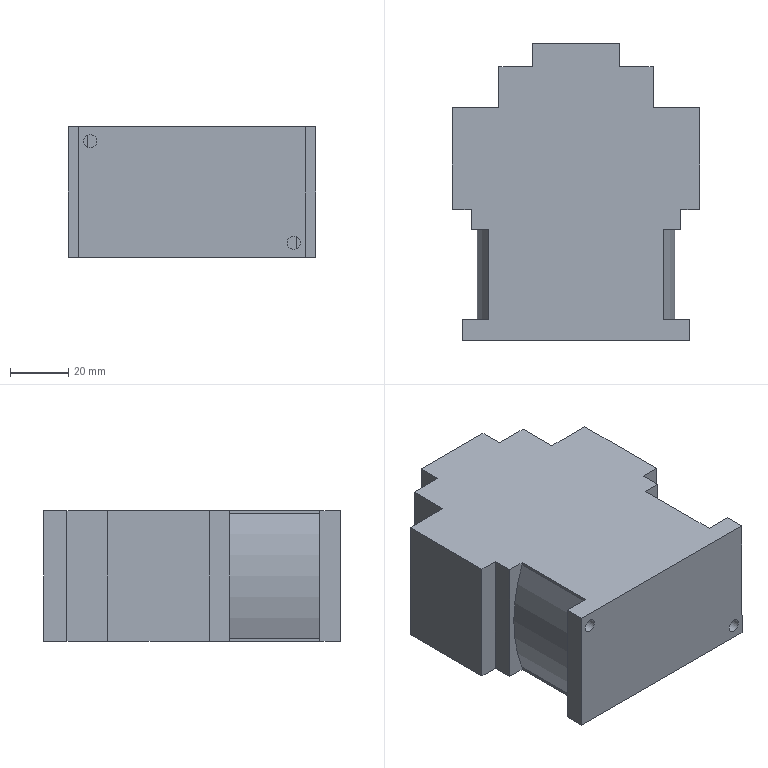Part | NX | features BREP 1 | 1 solid | 32 faces | box 85 x 102 x 45 mm | volume 315964 mm3 | plane 28 | cylinder 4 | commonest cylinder face diameters 4.5 x2 120 x2
STEP:
#1=CARTESIAN_POINT('',(-37.25,0.,17.5));
#2=VERTEX_POINT('',#1);
#3=CARTESIAN_POINT('',(-35.,0.,17.5));
#4=DIRECTION('',(0.,-1.,0.));
#5=DIRECTION('',(-1.,0.,0.));
#6=AXIS2_PLACEMENT_3D('',#3,#4,#5);
#7=CIRCLE('',#6,2.25);
#8=EDGE_CURVE('',#2,#2,#7,.T.);
#9=ORIENTED_EDGE('',*,*,#8,.T.);
#10=EDGE_LOOP('',(#9));
#11=FACE_BOUND('',#10,.T.);
#12=CARTESIAN_POINT('',(-32.75,7.,17.5));
#13=VERTEX_POINT('',#12);
#14=CARTESIAN_POINT('',(-35.,7.,17.5));
#15=DIRECTION('',(0.,-1.,0.));
#16=DIRECTION('',(1.,0.,0.));
#17=AXIS2_PLACEMENT_3D('',#14,#15,#16);
#18=CIRCLE('',#17,2.25);
#19=EDGE_CURVE('',#13,#13,#18,.T.);
#20=ORIENTED_EDGE('',*,*,#19,.F.);
#21=EDGE_LOOP('',(#20));
#22=FACE_BOUND('',#21,.T.);
#23=CARTESIAN_POINT('',(-35.,8.,17.5));
#24=DIRECTION('',(0.,-1.,0.));
#25=DIRECTION('',(1.,0.,0.));
#26=AXIS2_PLACEMENT_3D('',#23,#24,#25);
#27=CYLINDRICAL_SURFACE('',#26,2.25);
#28=ADVANCED_FACE('',(#11,#22),#27,.F.);
#29=CARTESIAN_POINT('',(32.75,0.,-17.5));
#30=VERTEX_POINT('',#29);
#31=CARTESIAN_POINT('',(35.,0.,-17.5));
#32=DIRECTION('',(0.,-1.,0.));
#33=DIRECTION('',(-1.,0.,0.));
#34=AXIS2_PLACEMENT_3D('',#31,#32,#33);
#35=CIRCLE('',#34,2.25);
#36=EDGE_CURVE('',#30,#30,#35,.T.);
#37=ORIENTED_EDGE('',*,*,#36,.T.);
#38=EDGE_LOOP('',(#37));
#39=FACE_BOUND('',#38,.T.);
#40=CARTESIAN_POINT('',(37.25,7.,-17.5));
#41=VERTEX_POINT('',#40);
#42=CARTESIAN_POINT('',(35.,7.,-17.5));
#43=DIRECTION('',(0.,-1.,0.));
#44=DIRECTION('',(1.,0.,0.));
#45=AXIS2_PLACEMENT_3D('',#42,#43,#44);
#46=CIRCLE('',#45,2.25);
#47=EDGE_CURVE('',#41,#41,#46,.T.);
#48=ORIENTED_EDGE('',*,*,#47,.F.);
#49=EDGE_LOOP('',(#48));
#50=FACE_BOUND('',#49,.T.);
#51=CARTESIAN_POINT('',(35.,8.,-17.5));
#52=DIRECTION('',(0.,-1.,0.));
#53=DIRECTION('',(1.,0.,0.));
#54=AXIS2_PLACEMENT_3D('',#51,#52,#53);
#55=CYLINDRICAL_SURFACE('',#54,2.25);
#56=ADVANCED_FACE('',(#39,#50),#55,.F.);
#57=CARTESIAN_POINT('',(30.,38.,21.541));
#58=VERTEX_POINT('',#57);
#59=CARTESIAN_POINT('',(30.,38.,-21.541));
#60=VERTEX_POINT('',#59);
#61=CARTESIAN_POINT('',(-26.,38.,0.));
#62=DIRECTION('',(0.,1.,0.));
#63=DIRECTION('',(0.,0.,1.));
#64=AXIS2_PLACEMENT_3D('',#61,#62,#63);
#65=CIRCLE('',#64,60.);
#66=EDGE_CURVE('',#58,#60,#65,.T.);
#67=ORIENTED_EDGE('',*,*,#66,.F.);
#68=CARTESIAN_POINT('',(30.,7.,21.541));
#69=VERTEX_POINT('',#68);
#70=CARTESIAN_POINT('',(30.,500000.,21.541));
#71=DIRECTION('',(0.,-1.,0.));
#72=VECTOR('',#71,1000.);
#73=LINE('',#70,#72);
#74=EDGE_CURVE('',#58,#69,#73,.T.);
#75=ORIENTED_EDGE('',*,*,#74,.T.);
#76=CARTESIAN_POINT('',(30.,7.,-21.541));
#77=VERTEX_POINT('',#76);
#78=CARTESIAN_POINT('',(-26.,7.,0.));
#79=DIRECTION('',(0.,1.,0.));
#80=DIRECTION('',(1.,0.,0.));
#81=AXIS2_PLACEMENT_3D('',#78,#79,#80);
#82=CIRCLE('',#81,60.);
#83=EDGE_CURVE('',#69,#77,#82,.T.);
#84=ORIENTED_EDGE('',*,*,#83,.T.);
#85=CARTESIAN_POINT('',(30.,500000.,-21.541));
#86=DIRECTION('',(0.,-1.,0.));
#87=VECTOR('',#86,1000.);
#88=LINE('',#85,#87);
#89=EDGE_CURVE('',#60,#77,#88,.T.);
#90=ORIENTED_EDGE('',*,*,#89,.F.);
#91=EDGE_LOOP('',(#67,#75,#84,#90));
#92=FACE_BOUND('',#91,.T.);
#93=CARTESIAN_POINT('',(-26.,500000.,0.));
#94=DIRECTION('',(0.,-1.,0.));
#95=DIRECTION('',(1.,0.,0.));
#96=AXIS2_PLACEMENT_3D('',#93,#94,#95);
#97=CYLINDRICAL_SURFACE('',#96,60.);
#98=ADVANCED_FACE('',(#92),#97,.T.);
#99=CARTESIAN_POINT('',(-30.,38.,-21.541));
#100=VERTEX_POINT('',#99);
#101=CARTESIAN_POINT('',(-30.,38.,21.541));
#102=VERTEX_POINT('',#101);
#103=CARTESIAN_POINT('',(26.,38.,0.));
#104=DIRECTION('',(0.,1.,0.));
#105=DIRECTION('',(0.,0.,1.));
#106=AXIS2_PLACEMENT_3D('',#103,#104,#105);
#107=CIRCLE('',#106,60.);
#108=EDGE_CURVE('',#100,#102,#107,.T.);
#109=ORIENTED_EDGE('',*,*,#108,.T.);
#110=CARTESIAN_POINT('',(-30.,38.,22.5));
#111=VERTEX_POINT('',#110);
#112=CARTESIAN_POINT('',(-30.,38.,22.5));
#113=DIRECTION('',(0.,0.,-1.));
#114=VECTOR('',#113,1000.);
#115=LINE('',#112,#114);
#116=EDGE_CURVE('',#111,#102,#115,.T.);
#117=ORIENTED_EDGE('',*,*,#116,.F.);
#118=CARTESIAN_POINT('',(-36.,38.,22.5));
#119=VERTEX_POINT('',#118);
#120=CARTESIAN_POINT('',(-30.,38.,22.5));
#121=DIRECTION('',(1.,0.,0.));
#122=VECTOR('',#121,1000.);
#123=LINE('',#120,#122);
#124=EDGE_CURVE('',#119,#111,#123,.T.);
#125=ORIENTED_EDGE('',*,*,#124,.F.);
#126=CARTESIAN_POINT('',(-36.,38.,-22.5));
#127=VERTEX_POINT('',#126);
#128=CARTESIAN_POINT('',(-36.,38.,22.5));
#129=DIRECTION('',(0.,0.,-1.));
#130=VECTOR('',#129,1000.);
#131=LINE('',#128,#130);
#132=EDGE_CURVE('',#119,#127,#131,.T.);
#133=ORIENTED_EDGE('',*,*,#132,.T.);
#134=CARTESIAN_POINT('',(-30.,38.,-22.5));
#135=VERTEX_POINT('',#134);
#136=CARTESIAN_POINT('',(-30.,38.,-22.5));
#137=DIRECTION('',(1.,0.,0.));
#138=VECTOR('',#137,1000.);
#139=LINE('',#136,#138);
#140=EDGE_CURVE('',#127,#135,#139,.T.);
#141=ORIENTED_EDGE('',*,*,#140,.T.);
#142=CARTESIAN_POINT('',(-30.,38.,22.5));
#143=DIRECTION('',(0.,0.,-1.));
#144=VECTOR('',#143,1000.);
#145=LINE('',#142,#144);
#146=EDGE_CURVE('',#100,#135,#145,.T.);
#147=ORIENTED_EDGE('',*,*,#146,.F.);
#148=EDGE_LOOP('',(#109,#117,#125,#133,#141,#147));
#149=FACE_BOUND('',#148,.T.);
#150=CARTESIAN_POINT('',(-30.,38.,22.5));
#151=DIRECTION('',(0.,1.,0.));
#152=DIRECTION('',(0.,0.,1.));
#153=AXIS2_PLACEMENT_3D('',#150,#151,#152);
#154=PLANE('',#153);
#155=ADVANCED_FACE('',(#149),#154,.F.);
#156=CARTESIAN_POINT('',(-30.,7.,21.541));
#157=VERTEX_POINT('',#156);
#158=CARTESIAN_POINT('',(-30.,500000.,21.541));
#159=DIRECTION('',(0.,-1.,0.));
#160=VECTOR('',#159,1000.);
#161=LINE('',#158,#160);
#162=EDGE_CURVE('',#102,#157,#161,.T.);
#163=ORIENTED_EDGE('',*,*,#162,.T.);
#164=CARTESIAN_POINT('',(-30.,7.,22.5));
#165=VERTEX_POINT('',#164);
#166=CARTESIAN_POINT('',(-30.,7.,22.5));
#167=DIRECTION('',(0.,0.,-1.));
#168=VECTOR('',#167,1000.);
#169=LINE('',#166,#168);
#170=EDGE_CURVE('',#165,#157,#169,.T.);
#171=ORIENTED_EDGE('',*,*,#170,.F.);
#172=CARTESIAN_POINT('',(-30.,7.,22.5));
#173=DIRECTION('',(0.,-1.,0.));
#174=VECTOR('',#173,1000.);
#175=LINE('',#172,#174);
#176=EDGE_CURVE('',#111,#165,#175,.T.);
#177=ORIENTED_EDGE('',*,*,#176,.F.);
#178=ORIENTED_EDGE('',*,*,#116,.T.);
#179=EDGE_LOOP('',(#163,#171,#177,#178));
#180=FACE_BOUND('',#179,.T.);
#181=CARTESIAN_POINT('',(-30.,7.,22.5));
#182=DIRECTION('',(1.,0.,0.));
#183=DIRECTION('',(0.,1.,0.));
#184=AXIS2_PLACEMENT_3D('',#181,#182,#183);
#185=PLANE('',#184);
#186=ADVANCED_FACE('',(#180),#185,.F.);
#187=CARTESIAN_POINT('',(-30.,7.,-21.541));
#188=VERTEX_POINT('',#187);
#189=CARTESIAN_POINT('',(-30.,500000.,-21.541));
#190=DIRECTION('',(0.,-1.,0.));
#191=VECTOR('',#190,1000.);
#192=LINE('',#189,#191);
#193=EDGE_CURVE('',#100,#188,#192,.T.);
#194=ORIENTED_EDGE('',*,*,#193,.F.);
#195=ORIENTED_EDGE('',*,*,#146,.T.);
#196=CARTESIAN_POINT('',(-30.,7.,-22.5));
#197=VERTEX_POINT('',#196);
#198=CARTESIAN_POINT('',(-30.,7.,-22.5));
#199=DIRECTION('',(0.,-1.,0.));
#200=VECTOR('',#199,1000.);
#201=LINE('',#198,#200);
#202=EDGE_CURVE('',#135,#197,#201,.T.);
#203=ORIENTED_EDGE('',*,*,#202,.T.);
#204=CARTESIAN_POINT('',(-30.,7.,22.5));
#205=DIRECTION('',(0.,0.,-1.));
#206=VECTOR('',#205,1000.);
#207=LINE('',#204,#206);
#208=EDGE_CURVE('',#188,#197,#207,.T.);
#209=ORIENTED_EDGE('',*,*,#208,.F.);
#210=EDGE_LOOP('',(#194,#195,#203,#209));
#211=FACE_BOUND('',#210,.T.);
#212=CARTESIAN_POINT('',(-30.,7.,22.5));
#213=DIRECTION('',(1.,0.,0.));
#214=DIRECTION('',(0.,1.,0.));
#215=AXIS2_PLACEMENT_3D('',#212,#213,#214);
#216=PLANE('',#215);
#217=ADVANCED_FACE('',(#211),#216,.F.);
#218=ORIENTED_EDGE('',*,*,#19,.T.);
#219=EDGE_LOOP('',(#218));
#220=FACE_BOUND('',#219,.T.);
#221=CARTESIAN_POINT('',(26.,7.,0.));
#222=DIRECTION('',(0.,1.,0.));
#223=DIRECTION('',(-1.,0.,0.));
#224=AXIS2_PLACEMENT_3D('',#221,#222,#223);
#225=CIRCLE('',#224,60.);
#226=EDGE_CURVE('',#188,#157,#225,.T.);
#227=ORIENTED_EDGE('',*,*,#226,.F.);
#228=ORIENTED_EDGE('',*,*,#208,.T.);
#229=CARTESIAN_POINT('',(-39.,7.,-22.5));
#230=VERTEX_POINT('',#229);
#231=CARTESIAN_POINT('',(-39.,7.,-22.5));
#232=DIRECTION('',(-1.,0.,0.));
#233=VECTOR('',#232,1000.);
#234=LINE('',#231,#233);
#235=EDGE_CURVE('',#197,#230,#234,.T.);
#236=ORIENTED_EDGE('',*,*,#235,.T.);
#237=CARTESIAN_POINT('',(-39.,7.,22.5));
#238=VERTEX_POINT('',#237);
#239=CARTESIAN_POINT('',(-39.,7.,22.5));
#240=DIRECTION('',(0.,0.,-1.));
#241=VECTOR('',#240,1000.);
#242=LINE('',#239,#241);
#243=EDGE_CURVE('',#238,#230,#242,.T.);
#244=ORIENTED_EDGE('',*,*,#243,.F.);
#245=CARTESIAN_POINT('',(-39.,7.,22.5));
#246=DIRECTION('',(-1.,0.,0.));
#247=VECTOR('',#246,1000.);
#248=LINE('',#245,#247);
#249=EDGE_CURVE('',#165,#238,#248,.T.);
#250=ORIENTED_EDGE('',*,*,#249,.F.);
#251=ORIENTED_EDGE('',*,*,#170,.T.);
#252=EDGE_LOOP('',(#227,#228,#236,#244,#250,#251));
#253=FACE_BOUND('',#252,.T.);
#254=CARTESIAN_POINT('',(-39.,7.,22.5));
#255=DIRECTION('',(0.,-1.,0.));
#256=DIRECTION('',(1.,0.,0.));
#257=AXIS2_PLACEMENT_3D('',#254,#255,#256);
#258=PLANE('',#257);
#259=ADVANCED_FACE('',(#220,#253),#258,.F.);
#260=ORIENTED_EDGE('',*,*,#47,.T.);
#261=EDGE_LOOP('',(#260));
#262=FACE_BOUND('',#261,.T.);
#263=ORIENTED_EDGE('',*,*,#83,.F.);
#264=CARTESIAN_POINT('',(30.,7.,22.5));
#265=VERTEX_POINT('',#264);
#266=CARTESIAN_POINT('',(30.,7.,22.5));
#267=DIRECTION('',(0.,0.,-1.));
#268=VECTOR('',#267,1000.);
#269=LINE('',#266,#268);
#270=EDGE_CURVE('',#265,#69,#269,.T.);
#271=ORIENTED_EDGE('',*,*,#270,.F.);
#272=CARTESIAN_POINT('',(39.,7.,22.5));
#273=VERTEX_POINT('',#272);
#274=CARTESIAN_POINT('',(39.,7.,22.5));
#275=DIRECTION('',(-1.,0.,0.));
#276=VECTOR('',#275,1000.);
#277=LINE('',#274,#276);
#278=EDGE_CURVE('',#273,#265,#277,.T.);
#279=ORIENTED_EDGE('',*,*,#278,.F.);
#280=CARTESIAN_POINT('',(39.,7.,-22.5));
#281=VERTEX_POINT('',#280);
#282=CARTESIAN_POINT('',(39.,7.,22.5));
#283=DIRECTION('',(0.,0.,-1.));
#284=VECTOR('',#283,1000.);
#285=LINE('',#282,#284);
#286=EDGE_CURVE('',#273,#281,#285,.T.);
#287=ORIENTED_EDGE('',*,*,#286,.T.);
#288=CARTESIAN_POINT('',(30.,7.,-22.5));
#289=VERTEX_POINT('',#288);
#290=CARTESIAN_POINT('',(39.,7.,-22.5));
#291=DIRECTION('',(-1.,0.,0.));
#292=VECTOR('',#291,1000.);
#293=LINE('',#290,#292);
#294=EDGE_CURVE('',#281,#289,#293,.T.);
#295=ORIENTED_EDGE('',*,*,#294,.T.);
#296=CARTESIAN_POINT('',(30.,7.,22.5));
#297=DIRECTION('',(0.,0.,-1.));
#298=VECTOR('',#297,1000.);
#299=LINE('',#296,#298);
#300=EDGE_CURVE('',#77,#289,#299,.T.);
#301=ORIENTED_EDGE('',*,*,#300,.F.);
#302=EDGE_LOOP('',(#263,#271,#279,#287,#295,#301));
#303=FACE_BOUND('',#302,.T.);
#304=CARTESIAN_POINT('',(39.,7.,22.5));
#305=DIRECTION('',(0.,-1.,0.));
#306=DIRECTION('',(1.,0.,0.));
#307=AXIS2_PLACEMENT_3D('',#304,#305,#306);
#308=PLANE('',#307);
#309=ADVANCED_FACE('',(#262,#303),#308,.F.);
#310=ORIENTED_EDGE('',*,*,#89,.T.);
#311=ORIENTED_EDGE('',*,*,#300,.T.);
#312=CARTESIAN_POINT('',(30.,38.,-22.5));
#313=VERTEX_POINT('',#312);
#314=CARTESIAN_POINT('',(30.,7.,-22.5));
#315=DIRECTION('',(0.,1.,0.));
#316=VECTOR('',#315,1000.);
#317=LINE('',#314,#316);
#318=EDGE_CURVE('',#289,#313,#317,.T.);
#319=ORIENTED_EDGE('',*,*,#318,.T.);
#320=CARTESIAN_POINT('',(30.,38.,22.5));
#321=DIRECTION('',(0.,0.,-1.));
#322=VECTOR('',#321,1000.);
#323=LINE('',#320,#322);
#324=EDGE_CURVE('',#60,#313,#323,.T.);
#325=ORIENTED_EDGE('',*,*,#324,.F.);
#326=EDGE_LOOP('',(#310,#311,#319,#325));
#327=FACE_BOUND('',#326,.T.);
#328=CARTESIAN_POINT('',(30.,7.,22.5));
#329=DIRECTION('',(-1.,0.,0.));
#330=DIRECTION('',(0.,0.,1.));
#331=AXIS2_PLACEMENT_3D('',#328,#329,#330);
#332=PLANE('',#331);
#333=ADVANCED_FACE('',(#327),#332,.F.);
#334=ORIENTED_EDGE('',*,*,#74,.F.);
#335=CARTESIAN_POINT('',(30.,38.,22.5));
#336=VERTEX_POINT('',#335);
#337=CARTESIAN_POINT('',(30.,38.,22.5));
#338=DIRECTION('',(0.,0.,-1.));
#339=VECTOR('',#338,1000.);
#340=LINE('',#337,#339);
#341=EDGE_CURVE('',#336,#58,#340,.T.);
#342=ORIENTED_EDGE('',*,*,#341,.F.);
#343=CARTESIAN_POINT('',(30.,7.,22.5));
#344=DIRECTION('',(0.,1.,0.));
#345=VECTOR('',#344,1000.);
#346=LINE('',#343,#345);
#347=EDGE_CURVE('',#265,#336,#346,.T.);
#348=ORIENTED_EDGE('',*,*,#347,.F.);
#349=ORIENTED_EDGE('',*,*,#270,.T.);
#350=EDGE_LOOP('',(#334,#342,#348,#349));
#351=FACE_BOUND('',#350,.T.);
#352=CARTESIAN_POINT('',(30.,7.,22.5));
#353=DIRECTION('',(-1.,0.,0.));
#354=DIRECTION('',(0.,0.,1.));
#355=AXIS2_PLACEMENT_3D('',#352,#353,#354);
#356=PLANE('',#355);
#357=ADVANCED_FACE('',(#351),#356,.F.);
#358=ORIENTED_EDGE('',*,*,#341,.T.);
#359=ORIENTED_EDGE('',*,*,#66,.T.);
#360=ORIENTED_EDGE('',*,*,#324,.T.);
#361=CARTESIAN_POINT('',(36.,38.,-22.5));
#362=VERTEX_POINT('',#361);
#363=CARTESIAN_POINT('',(30.,38.,-22.5));
#364=DIRECTION('',(1.,0.,0.));
#365=VECTOR('',#364,1000.);
#366=LINE('',#363,#365);
#367=EDGE_CURVE('',#313,#362,#366,.T.);
#368=ORIENTED_EDGE('',*,*,#367,.T.);
#369=CARTESIAN_POINT('',(36.,38.,22.5));
#370=VERTEX_POINT('',#369);
#371=CARTESIAN_POINT('',(36.,38.,22.5));
#372=DIRECTION('',(0.,0.,-1.));
#373=VECTOR('',#372,1000.);
#374=LINE('',#371,#373);
#375=EDGE_CURVE('',#370,#362,#374,.T.);
#376=ORIENTED_EDGE('',*,*,#375,.F.);
#377=CARTESIAN_POINT('',(30.,38.,22.5));
#378=DIRECTION('',(1.,0.,0.));
#379=VECTOR('',#378,1000.);
#380=LINE('',#377,#379);
#381=EDGE_CURVE('',#336,#370,#380,.T.);
#382=ORIENTED_EDGE('',*,*,#381,.F.);
#383=EDGE_LOOP('',(#358,#359,#360,#368,#376,#382));
#384=FACE_BOUND('',#383,.T.);
#385=CARTESIAN_POINT('',(30.,38.,22.5));
#386=DIRECTION('',(0.,1.,0.));
#387=DIRECTION('',(0.,0.,1.));
#388=AXIS2_PLACEMENT_3D('',#385,#386,#387);
#389=PLANE('',#388);
#390=ADVANCED_FACE('',(#384),#389,.F.);
#391=CARTESIAN_POINT('',(39.,0.,-22.5));
#392=VERTEX_POINT('',#391);
#393=CARTESIAN_POINT('',(39.,0.,-22.5));
#394=DIRECTION('',(0.,1.,0.));
#395=VECTOR('',#394,1000.);
#396=LINE('',#393,#395);
#397=EDGE_CURVE('',#392,#281,#396,.T.);
#398=ORIENTED_EDGE('',*,*,#397,.T.);
#399=ORIENTED_EDGE('',*,*,#286,.F.);
#400=CARTESIAN_POINT('',(39.,0.,22.5));
#401=VERTEX_POINT('',#400);
#402=CARTESIAN_POINT('',(39.,0.,22.5));
#403=DIRECTION('',(0.,1.,0.));
#404=VECTOR('',#403,1000.);
#405=LINE('',#402,#404);
#406=EDGE_CURVE('',#401,#273,#405,.T.);
#407=ORIENTED_EDGE('',*,*,#406,.F.);
#408=CARTESIAN_POINT('',(39.,0.,22.5));
#409=DIRECTION('',(0.,0.,-1.));
#410=VECTOR('',#409,1000.);
#411=LINE('',#408,#410);
#412=EDGE_CURVE('',#401,#392,#411,.T.);
#413=ORIENTED_EDGE('',*,*,#412,.T.);
#414=EDGE_LOOP('',(#398,#399,#407,#413));
#415=FACE_BOUND('',#414,.T.);
#416=CARTESIAN_POINT('',(39.,0.,22.5));
#417=DIRECTION('',(-1.,0.,0.));
#418=DIRECTION('',(0.,0.,1.));
#419=AXIS2_PLACEMENT_3D('',#416,#417,#418);
#420=PLANE('',#419);
#421=ADVANCED_FACE('',(#415),#420,.F.);
#422=CARTESIAN_POINT('',(36.,45.,-22.5));
#423=VERTEX_POINT('',#422);
#424=CARTESIAN_POINT('',(36.,38.,-22.5));
#425=DIRECTION('',(0.,1.,0.));
#426=VECTOR('',#425,1000.);
#427=LINE('',#424,#426);
#428=EDGE_CURVE('',#362,#423,#427,.T.);
#429=ORIENTED_EDGE('',*,*,#428,.T.);
#430=CARTESIAN_POINT('',(36.,45.,22.5));
#431=VERTEX_POINT('',#430);
#432=CARTESIAN_POINT('',(36.,45.,22.5));
#433=DIRECTION('',(0.,0.,-1.));
#434=VECTOR('',#433,1000.);
#435=LINE('',#432,#434);
#436=EDGE_CURVE('',#431,#423,#435,.T.);
#437=ORIENTED_EDGE('',*,*,#436,.F.);
#438=CARTESIAN_POINT('',(36.,38.,22.5));
#439=DIRECTION('',(0.,1.,0.));
#440=VECTOR('',#439,1000.);
#441=LINE('',#438,#440);
#442=EDGE_CURVE('',#370,#431,#441,.T.);
#443=ORIENTED_EDGE('',*,*,#442,.F.);
#444=ORIENTED_EDGE('',*,*,#375,.T.);
#445=EDGE_LOOP('',(#429,#437,#443,#444));
#446=FACE_BOUND('',#445,.T.);
#447=CARTESIAN_POINT('',(36.,38.,22.5));
#448=DIRECTION('',(-1.,0.,0.));
#449=DIRECTION('',(0.,0.,1.));
#450=AXIS2_PLACEMENT_3D('',#447,#448,#449);
#451=PLANE('',#450);
#452=ADVANCED_FACE('',(#446),#451,.F.);
#453=CARTESIAN_POINT('',(42.5,45.,-22.5));
#454=VERTEX_POINT('',#453);
#455=CARTESIAN_POINT('',(36.,45.,-22.5));
#456=DIRECTION('',(1.,0.,0.));
#457=VECTOR('',#456,1000.);
#458=LINE('',#455,#457);
#459=EDGE_CURVE('',#423,#454,#458,.T.);
#460=ORIENTED_EDGE('',*,*,#459,.T.);
#461=CARTESIAN_POINT('',(42.5,45.,22.5));
#462=VERTEX_POINT('',#461);
#463=CARTESIAN_POINT('',(42.5,45.,22.5));
#464=DIRECTION('',(0.,0.,-1.));
#465=VECTOR('',#464,1000.);
#466=LINE('',#463,#465);
#467=EDGE_CURVE('',#462,#454,#466,.T.);
#468=ORIENTED_EDGE('',*,*,#467,.F.);
#469=CARTESIAN_POINT('',(36.,45.,22.5));
#470=DIRECTION('',(1.,0.,0.));
#471=VECTOR('',#470,1000.);
#472=LINE('',#469,#471);
#473=EDGE_CURVE('',#431,#462,#472,.T.);
#474=ORIENTED_EDGE('',*,*,#473,.F.);
#475=ORIENTED_EDGE('',*,*,#436,.T.);
#476=EDGE_LOOP('',(#460,#468,#474,#475));
#477=FACE_BOUND('',#476,.T.);
#478=CARTESIAN_POINT('',(36.,45.,22.5));
#479=DIRECTION('',(0.,1.,0.));
#480=DIRECTION('',(-1.,0.,0.));
#481=AXIS2_PLACEMENT_3D('',#478,#479,#480);
#482=PLANE('',#481);
#483=ADVANCED_FACE('',(#477),#482,.F.);
#484=CARTESIAN_POINT('',(42.5,80.,-22.5));
#485=VERTEX_POINT('',#484);
#486=CARTESIAN_POINT('',(42.5,45.,-22.5));
#487=DIRECTION('',(0.,1.,0.));
#488=VECTOR('',#487,1000.);
#489=LINE('',#486,#488);
#490=EDGE_CURVE('',#454,#485,#489,.T.);
#491=ORIENTED_EDGE('',*,*,#490,.T.);
#492=CARTESIAN_POINT('',(42.5,80.,22.5));
#493=VERTEX_POINT('',#492);
#494=CARTESIAN_POINT('',(42.5,80.,22.5));
#495=DIRECTION('',(0.,0.,-1.));
#496=VECTOR('',#495,1000.);
#497=LINE('',#494,#496);
#498=EDGE_CURVE('',#493,#485,#497,.T.);
#499=ORIENTED_EDGE('',*,*,#498,.F.);
#500=CARTESIAN_POINT('',(42.5,45.,22.5));
#501=DIRECTION('',(0.,1.,0.));
#502=VECTOR('',#501,1000.);
#503=LINE('',#500,#502);
#504=EDGE_CURVE('',#462,#493,#503,.T.);
#505=ORIENTED_EDGE('',*,*,#504,.F.);
#506=ORIENTED_EDGE('',*,*,#467,.T.);
#507=EDGE_LOOP('',(#491,#499,#505,#506));
#508=FACE_BOUND('',#507,.T.);
#509=CARTESIAN_POINT('',(42.5,45.,22.5));
#510=DIRECTION('',(-1.,0.,0.));
#511=DIRECTION('',(0.,0.,1.));
#512=AXIS2_PLACEMENT_3D('',#509,#510,#511);
#513=PLANE('',#512);
#514=ADVANCED_FACE('',(#508),#513,.F.);
#515=CARTESIAN_POINT('',(26.5,80.,-22.5));
#516=VERTEX_POINT('',#515);
#517=CARTESIAN_POINT('',(42.5,80.,-22.5));
#518=DIRECTION('',(-1.,0.,0.));
#519=VECTOR('',#518,1000.);
#520=LINE('',#517,#519);
#521=EDGE_CURVE('',#485,#516,#520,.T.);
#522=ORIENTED_EDGE('',*,*,#521,.T.);
#523=CARTESIAN_POINT('',(26.5,80.,22.5));
#524=VERTEX_POINT('',#523);
#525=CARTESIAN_POINT('',(26.5,80.,22.5));
#526=DIRECTION('',(0.,0.,-1.));
#527=VECTOR('',#526,1000.);
#528=LINE('',#525,#527);
#529=EDGE_CURVE('',#524,#516,#528,.T.);
#530=ORIENTED_EDGE('',*,*,#529,.F.);
#531=CARTESIAN_POINT('',(42.5,80.,22.5));
#532=DIRECTION('',(-1.,0.,0.));
#533=VECTOR('',#532,1000.);
#534=LINE('',#531,#533);
#535=EDGE_CURVE('',#493,#524,#534,.T.);
#536=ORIENTED_EDGE('',*,*,#535,.F.);
#537=ORIENTED_EDGE('',*,*,#498,.T.);
#538=EDGE_LOOP('',(#522,#530,#536,#537));
#539=FACE_BOUND('',#538,.T.);
#540=CARTESIAN_POINT('',(42.5,80.,22.5));
#541=DIRECTION('',(0.,-1.,0.));
#542=DIRECTION('',(1.,0.,0.));
#543=AXIS2_PLACEMENT_3D('',#540,#541,#542);
#544=PLANE('',#543);
#545=ADVANCED_FACE('',(#539),#544,.F.);
#546=CARTESIAN_POINT('',(26.5,94.,-22.5));
#547=VERTEX_POINT('',#546);
#548=CARTESIAN_POINT('',(26.5,80.,-22.5));
#549=DIRECTION('',(0.,1.,0.));
#550=VECTOR('',#549,1000.);
#551=LINE('',#548,#550);
#552=EDGE_CURVE('',#516,#547,#551,.T.);
#553=ORIENTED_EDGE('',*,*,#552,.T.);
#554=CARTESIAN_POINT('',(26.5,94.,22.5));
#555=VERTEX_POINT('',#554);
#556=CARTESIAN_POINT('',(26.5,94.,22.5));
#557=DIRECTION('',(0.,0.,-1.));
#558=VECTOR('',#557,1000.);
#559=LINE('',#556,#558);
#560=EDGE_CURVE('',#555,#547,#559,.T.);
#561=ORIENTED_EDGE('',*,*,#560,.F.);
#562=CARTESIAN_POINT('',(26.5,80.,22.5));
#563=DIRECTION('',(0.,1.,0.));
#564=VECTOR('',#563,1000.);
#565=LINE('',#562,#564);
#566=EDGE_CURVE('',#524,#555,#565,.T.);
#567=ORIENTED_EDGE('',*,*,#566,.F.);
#568=ORIENTED_EDGE('',*,*,#529,.T.);
#569=EDGE_LOOP('',(#553,#561,#567,#568));
#570=FACE_BOUND('',#569,.T.);
#571=CARTESIAN_POINT('',(26.5,80.,22.5));
#572=DIRECTION('',(-1.,0.,0.));
#573=DIRECTION('',(0.,0.,1.));
#574=AXIS2_PLACEMENT_3D('',#571,#572,#573);
#575=PLANE('',#574);
#576=ADVANCED_FACE('',(#570),#575,.F.);
#577=CARTESIAN_POINT('',(15.,94.,-22.5));
#578=VERTEX_POINT('',#577);
#579=CARTESIAN_POINT('',(26.5,94.,-22.5));
#580=DIRECTION('',(-1.,0.,0.));
#581=VECTOR('',#580,1000.);
#582=LINE('',#579,#581);
#583=EDGE_CURVE('',#547,#578,#582,.T.);
#584=ORIENTED_EDGE('',*,*,#583,.T.);
#585=CARTESIAN_POINT('',(15.,94.,22.5));
#586=VERTEX_POINT('',#585);
#587=CARTESIAN_POINT('',(15.,94.,22.5));
#588=DIRECTION('',(0.,0.,-1.));
#589=VECTOR('',#588,1000.);
#590=LINE('',#587,#589);
#591=EDGE_CURVE('',#586,#578,#590,.T.);
#592=ORIENTED_EDGE('',*,*,#591,.F.);
#593=CARTESIAN_POINT('',(26.5,94.,22.5));
#594=DIRECTION('',(-1.,0.,0.));
#595=VECTOR('',#594,1000.);
#596=LINE('',#593,#595);
#597=EDGE_CURVE('',#555,#586,#596,.T.);
#598=ORIENTED_EDGE('',*,*,#597,.F.);
#599=ORIENTED_EDGE('',*,*,#560,.T.);
#600=EDGE_LOOP('',(#584,#592,#598,#599));
#601=FACE_BOUND('',#600,.T.);
#602=CARTESIAN_POINT('',(26.5,94.,22.5));
#603=DIRECTION('',(0.,-1.,0.));
#604=DIRECTION('',(0.,0.,-1.));
#605=AXIS2_PLACEMENT_3D('',#602,#603,#604);
#606=PLANE('',#605);
#607=ADVANCED_FACE('',(#601),#606,.F.);
#608=CARTESIAN_POINT('',(15.,102.,-22.5));
#609=VERTEX_POINT('',#608);
#610=CARTESIAN_POINT('',(15.,94.,-22.5));
#611=DIRECTION('',(0.,1.,0.));
#612=VECTOR('',#611,1000.);
#613=LINE('',#610,#612);
#614=EDGE_CURVE('',#578,#609,#613,.T.);
#615=ORIENTED_EDGE('',*,*,#614,.T.);
#616=CARTESIAN_POINT('',(15.,102.,22.5));
#617=VERTEX_POINT('',#616);
#618=CARTESIAN_POINT('',(15.,102.,22.5));
#619=DIRECTION('',(0.,0.,-1.));
#620=VECTOR('',#619,1000.);
#621=LINE('',#618,#620);
#622=EDGE_CURVE('',#617,#609,#621,.T.);
#623=ORIENTED_EDGE('',*,*,#622,.F.);
#624=CARTESIAN_POINT('',(15.,94.,22.5));
#625=DIRECTION('',(0.,1.,0.));
#626=VECTOR('',#625,1000.);
#627=LINE('',#624,#626);
#628=EDGE_CURVE('',#586,#617,#627,.T.);
#629=ORIENTED_EDGE('',*,*,#628,.F.);
#630=ORIENTED_EDGE('',*,*,#591,.T.);
#631=EDGE_LOOP('',(#615,#623,#629,#630));
#632=FACE_BOUND('',#631,.T.);
#633=CARTESIAN_POINT('',(15.,94.,22.5));
#634=DIRECTION('',(-1.,0.,0.));
#635=DIRECTION('',(0.,-1.,0.));
#636=AXIS2_PLACEMENT_3D('',#633,#634,#635);
#637=PLANE('',#636);
#638=ADVANCED_FACE('',(#632),#637,.F.);
#639=CARTESIAN_POINT('',(-15.,102.,-22.5));
#640=VERTEX_POINT('',#639);
#641=CARTESIAN_POINT('',(15.,102.,-22.5));
#642=DIRECTION('',(-1.,0.,0.));
#643=VECTOR('',#642,1000.);
#644=LINE('',#641,#643);
#645=EDGE_CURVE('',#609,#640,#644,.T.);
#646=ORIENTED_EDGE('',*,*,#645,.T.);
#647=CARTESIAN_POINT('',(-15.,102.,22.5));
#648=VERTEX_POINT('',#647);
#649=CARTESIAN_POINT('',(-15.,102.,22.5));
#650=DIRECTION('',(0.,0.,-1.));
#651=VECTOR('',#650,1000.);
#652=LINE('',#649,#651);
#653=EDGE_CURVE('',#648,#640,#652,.T.);
#654=ORIENTED_EDGE('',*,*,#653,.F.);
#655=CARTESIAN_POINT('',(15.,102.,22.5));
#656=DIRECTION('',(-1.,0.,0.));
#657=VECTOR('',#656,1000.);
#658=LINE('',#655,#657);
#659=EDGE_CURVE('',#617,#648,#658,.T.);
#660=ORIENTED_EDGE('',*,*,#659,.F.);
#661=ORIENTED_EDGE('',*,*,#622,.T.);
#662=EDGE_LOOP('',(#646,#654,#660,#661));
#663=FACE_BOUND('',#662,.T.);
#664=CARTESIAN_POINT('',(15.,102.,22.5));
#665=DIRECTION('',(0.,-1.,0.));
#666=DIRECTION('',(0.,0.,-1.));
#667=AXIS2_PLACEMENT_3D('',#664,#665,#666);
#668=PLANE('',#667);
#669=ADVANCED_FACE('',(#663),#668,.F.);
#670=CARTESIAN_POINT('',(-15.,94.,-22.5));
#671=VERTEX_POINT('',#670);
#672=CARTESIAN_POINT('',(-15.,94.,-22.5));
#673=DIRECTION('',(0.,-1.,0.));
#674=VECTOR('',#673,1000.);
#675=LINE('',#672,#674);
#676=EDGE_CURVE('',#640,#671,#675,.T.);
#677=ORIENTED_EDGE('',*,*,#676,.T.);
#678=CARTESIAN_POINT('',(-15.,94.,22.5));
#679=VERTEX_POINT('',#678);
#680=CARTESIAN_POINT('',(-15.,94.,22.5));
#681=DIRECTION('',(0.,0.,-1.));
#682=VECTOR('',#681,1000.);
#683=LINE('',#680,#682);
#684=EDGE_CURVE('',#679,#671,#683,.T.);
#685=ORIENTED_EDGE('',*,*,#684,.F.);
#686=CARTESIAN_POINT('',(-15.,94.,22.5));
#687=DIRECTION('',(0.,-1.,0.));
#688=VECTOR('',#687,1000.);
#689=LINE('',#686,#688);
#690=EDGE_CURVE('',#648,#679,#689,.T.);
#691=ORIENTED_EDGE('',*,*,#690,.F.);
#692=ORIENTED_EDGE('',*,*,#653,.T.);
#693=EDGE_LOOP('',(#677,#685,#691,#692));
#694=FACE_BOUND('',#693,.T.);
#695=CARTESIAN_POINT('',(-15.,94.,22.5));
#696=DIRECTION('',(1.,0.,0.));
#697=DIRECTION('',(0.,1.,0.));
#698=AXIS2_PLACEMENT_3D('',#695,#696,#697);
#699=PLANE('',#698);
#700=ADVANCED_FACE('',(#694),#699,.F.);
#701=CARTESIAN_POINT('',(-26.5,94.,-22.5));
#702=VERTEX_POINT('',#701);
#703=CARTESIAN_POINT('',(-26.5,94.,-22.5));
#704=DIRECTION('',(-1.,0.,0.));
#705=VECTOR('',#704,1000.);
#706=LINE('',#703,#705);
#707=EDGE_CURVE('',#671,#702,#706,.T.);
#708=ORIENTED_EDGE('',*,*,#707,.T.);
#709=CARTESIAN_POINT('',(-26.5,94.,22.5));
#710=VERTEX_POINT('',#709);
#711=CARTESIAN_POINT('',(-26.5,94.,22.5));
#712=DIRECTION('',(0.,0.,-1.));
#713=VECTOR('',#712,1000.);
#714=LINE('',#711,#713);
#715=EDGE_CURVE('',#710,#702,#714,.T.);
#716=ORIENTED_EDGE('',*,*,#715,.F.);
#717=CARTESIAN_POINT('',(-26.5,94.,22.5));
#718=DIRECTION('',(-1.,0.,0.));
#719=VECTOR('',#718,1000.);
#720=LINE('',#717,#719);
#721=EDGE_CURVE('',#679,#710,#720,.T.);
#722=ORIENTED_EDGE('',*,*,#721,.F.);
#723=ORIENTED_EDGE('',*,*,#684,.T.);
#724=EDGE_LOOP('',(#708,#716,#722,#723));
#725=FACE_BOUND('',#724,.T.);
#726=CARTESIAN_POINT('',(-26.5,94.,22.5));
#727=DIRECTION('',(0.,-1.,0.));
#728=DIRECTION('',(0.,0.,-1.));
#729=AXIS2_PLACEMENT_3D('',#726,#727,#728);
#730=PLANE('',#729);
#731=ADVANCED_FACE('',(#725),#730,.F.);
#732=CARTESIAN_POINT('',(-26.5,80.,-22.5));
#733=VERTEX_POINT('',#732);
#734=CARTESIAN_POINT('',(-26.5,80.,-22.5));
#735=DIRECTION('',(0.,-1.,0.));
#736=VECTOR('',#735,1000.);
#737=LINE('',#734,#736);
#738=EDGE_CURVE('',#702,#733,#737,.T.);
#739=ORIENTED_EDGE('',*,*,#738,.T.);
#740=CARTESIAN_POINT('',(-26.5,80.,22.5));
#741=VERTEX_POINT('',#740);
#742=CARTESIAN_POINT('',(-26.5,80.,22.5));
#743=DIRECTION('',(0.,0.,-1.));
#744=VECTOR('',#743,1000.);
#745=LINE('',#742,#744);
#746=EDGE_CURVE('',#741,#733,#745,.T.);
#747=ORIENTED_EDGE('',*,*,#746,.F.);
#748=CARTESIAN_POINT('',(-26.5,80.,22.5));
#749=DIRECTION('',(0.,-1.,0.));
#750=VECTOR('',#749,1000.);
#751=LINE('',#748,#750);
#752=EDGE_CURVE('',#710,#741,#751,.T.);
#753=ORIENTED_EDGE('',*,*,#752,.F.);
#754=ORIENTED_EDGE('',*,*,#715,.T.);
#755=EDGE_LOOP('',(#739,#747,#753,#754));
#756=FACE_BOUND('',#755,.T.);
#757=CARTESIAN_POINT('',(-26.5,80.,22.5));
#758=DIRECTION('',(1.,0.,0.));
#759=DIRECTION('',(0.,0.,-1.));
#760=AXIS2_PLACEMENT_3D('',#757,#758,#759);
#761=PLANE('',#760);
#762=ADVANCED_FACE('',(#756),#761,.F.);
#763=CARTESIAN_POINT('',(-42.5,80.,-22.5));
#764=VERTEX_POINT('',#763);
#765=CARTESIAN_POINT('',(-42.5,80.,-22.5));
#766=DIRECTION('',(-1.,0.,0.));
#767=VECTOR('',#766,1000.);
#768=LINE('',#765,#767);
#769=EDGE_CURVE('',#733,#764,#768,.T.);
#770=ORIENTED_EDGE('',*,*,#769,.T.);
#771=CARTESIAN_POINT('',(-42.5,80.,22.5));
#772=VERTEX_POINT('',#771);
#773=CARTESIAN_POINT('',(-42.5,80.,22.5));
#774=DIRECTION('',(0.,0.,-1.));
#775=VECTOR('',#774,1000.);
#776=LINE('',#773,#775);
#777=EDGE_CURVE('',#772,#764,#776,.T.);
#778=ORIENTED_EDGE('',*,*,#777,.F.);
#779=CARTESIAN_POINT('',(-42.5,80.,22.5));
#780=DIRECTION('',(-1.,0.,0.));
#781=VECTOR('',#780,1000.);
#782=LINE('',#779,#781);
#783=EDGE_CURVE('',#741,#772,#782,.T.);
#784=ORIENTED_EDGE('',*,*,#783,.F.);
#785=ORIENTED_EDGE('',*,*,#746,.T.);
#786=EDGE_LOOP('',(#770,#778,#784,#785));
#787=FACE_BOUND('',#786,.T.);
#788=CARTESIAN_POINT('',(-42.5,80.,22.5));
#789=DIRECTION('',(0.,-1.,0.));
#790=DIRECTION('',(0.,0.,-1.));
#791=AXIS2_PLACEMENT_3D('',#788,#789,#790);
#792=PLANE('',#791);
#793=ADVANCED_FACE('',(#787),#792,.F.);
#794=CARTESIAN_POINT('',(-42.5,45.,-22.5));
#795=VERTEX_POINT('',#794);
#796=CARTESIAN_POINT('',(-42.5,45.,-22.5));
#797=DIRECTION('',(0.,-1.,0.));
#798=VECTOR('',#797,1000.);
#799=LINE('',#796,#798);
#800=EDGE_CURVE('',#764,#795,#799,.T.);
#801=ORIENTED_EDGE('',*,*,#800,.T.);
#802=CARTESIAN_POINT('',(-42.5,45.,22.5));
#803=VERTEX_POINT('',#802);
#804=CARTESIAN_POINT('',(-42.5,45.,22.5));
#805=DIRECTION('',(0.,0.,-1.));
#806=VECTOR('',#805,1000.);
#807=LINE('',#804,#806);
#808=EDGE_CURVE('',#803,#795,#807,.T.);
#809=ORIENTED_EDGE('',*,*,#808,.F.);
#810=CARTESIAN_POINT('',(-42.5,45.,22.5));
#811=DIRECTION('',(0.,-1.,0.));
#812=VECTOR('',#811,1000.);
#813=LINE('',#810,#812);
#814=EDGE_CURVE('',#772,#803,#813,.T.);
#815=ORIENTED_EDGE('',*,*,#814,.F.);
#816=ORIENTED_EDGE('',*,*,#777,.T.);
#817=EDGE_LOOP('',(#801,#809,#815,#816));
#818=FACE_BOUND('',#817,.T.);
#819=CARTESIAN_POINT('',(-42.5,45.,22.5));
#820=DIRECTION('',(1.,0.,0.));
#821=DIRECTION('',(0.,0.,-1.));
#822=AXIS2_PLACEMENT_3D('',#819,#820,#821);
#823=PLANE('',#822);
#824=ADVANCED_FACE('',(#818),#823,.F.);
#825=CARTESIAN_POINT('',(-36.,45.,-22.5));
#826=VERTEX_POINT('',#825);
#827=CARTESIAN_POINT('',(-36.,45.,-22.5));
#828=DIRECTION('',(1.,0.,0.));
#829=VECTOR('',#828,1000.);
#830=LINE('',#827,#829);
#831=EDGE_CURVE('',#795,#826,#830,.T.);
#832=ORIENTED_EDGE('',*,*,#831,.T.);
#833=CARTESIAN_POINT('',(-36.,45.,22.5));
#834=VERTEX_POINT('',#833);
#835=CARTESIAN_POINT('',(-36.,45.,22.5));
#836=DIRECTION('',(0.,0.,-1.));
#837=VECTOR('',#836,1000.);
#838=LINE('',#835,#837);
#839=EDGE_CURVE('',#834,#826,#838,.T.);
#840=ORIENTED_EDGE('',*,*,#839,.F.);
#841=CARTESIAN_POINT('',(-36.,45.,22.5));
#842=DIRECTION('',(1.,0.,0.));
#843=VECTOR('',#842,1000.);
#844=LINE('',#841,#843);
#845=EDGE_CURVE('',#803,#834,#844,.T.);
#846=ORIENTED_EDGE('',*,*,#845,.F.);
#847=ORIENTED_EDGE('',*,*,#808,.T.);
#848=EDGE_LOOP('',(#832,#840,#846,#847));
#849=FACE_BOUND('',#848,.T.);
#850=CARTESIAN_POINT('',(-36.,45.,22.5));
#851=DIRECTION('',(0.,1.,0.));
#852=DIRECTION('',(0.,0.,1.));
#853=AXIS2_PLACEMENT_3D('',#850,#851,#852);
#854=PLANE('',#853);
#855=ADVANCED_FACE('',(#849),#854,.F.);
#856=CARTESIAN_POINT('',(-36.,38.,-22.5));
#857=DIRECTION('',(0.,-1.,0.));
#858=VECTOR('',#857,1000.);
#859=LINE('',#856,#858);
#860=EDGE_CURVE('',#826,#127,#859,.T.);
#861=ORIENTED_EDGE('',*,*,#860,.T.);
#862=ORIENTED_EDGE('',*,*,#132,.F.);
#863=CARTESIAN_POINT('',(-36.,38.,22.5));
#864=DIRECTION('',(0.,-1.,0.));
#865=VECTOR('',#864,1000.);
#866=LINE('',#863,#865);
#867=EDGE_CURVE('',#834,#119,#866,.T.);
#868=ORIENTED_EDGE('',*,*,#867,.F.);
#869=ORIENTED_EDGE('',*,*,#839,.T.);
#870=EDGE_LOOP('',(#861,#862,#868,#869));
#871=FACE_BOUND('',#870,.T.);
#872=CARTESIAN_POINT('',(-36.,38.,22.5));
#873=DIRECTION('',(1.,0.,0.));
#874=DIRECTION('',(0.,0.,-1.));
#875=AXIS2_PLACEMENT_3D('',#872,#873,#874);
#876=PLANE('',#875);
#877=ADVANCED_FACE('',(#871),#876,.F.);
#878=CARTESIAN_POINT('',(-39.,0.,-22.5));
#879=VERTEX_POINT('',#878);
#880=CARTESIAN_POINT('',(-39.,0.,-22.5));
#881=DIRECTION('',(0.,-1.,0.));
#882=VECTOR('',#881,1000.);
#883=LINE('',#880,#882);
#884=EDGE_CURVE('',#230,#879,#883,.T.);
#885=ORIENTED_EDGE('',*,*,#884,.T.);
#886=CARTESIAN_POINT('',(-39.,0.,22.5));
#887=VERTEX_POINT('',#886);
#888=CARTESIAN_POINT('',(-39.,0.,22.5));
#889=DIRECTION('',(0.,0.,-1.));
#890=VECTOR('',#889,1000.);
#891=LINE('',#888,#890);
#892=EDGE_CURVE('',#887,#879,#891,.T.);
#893=ORIENTED_EDGE('',*,*,#892,.F.);
#894=CARTESIAN_POINT('',(-39.,0.,22.5));
#895=DIRECTION('',(0.,-1.,0.));
#896=VECTOR('',#895,1000.);
#897=LINE('',#894,#896);
#898=EDGE_CURVE('',#238,#887,#897,.T.);
#899=ORIENTED_EDGE('',*,*,#898,.F.);
#900=ORIENTED_EDGE('',*,*,#243,.T.);
#901=EDGE_LOOP('',(#885,#893,#899,#900));
#902=FACE_BOUND('',#901,.T.);
#903=CARTESIAN_POINT('',(-39.,0.,22.5));
#904=DIRECTION('',(1.,0.,0.));
#905=DIRECTION('',(0.,0.,-1.));
#906=AXIS2_PLACEMENT_3D('',#903,#904,#905);
#907=PLANE('',#906);
#908=ADVANCED_FACE('',(#902),#907,.F.);
#909=ORIENTED_EDGE('',*,*,#8,.F.);
#910=EDGE_LOOP('',(#909));
#911=FACE_BOUND('',#910,.T.);
#912=ORIENTED_EDGE('',*,*,#36,.F.);
#913=EDGE_LOOP('',(#912));
#914=FACE_BOUND('',#913,.T.);
#915=CARTESIAN_POINT('',(-39.,0.,-22.5));
#916=DIRECTION('',(1.,0.,0.));
#917=VECTOR('',#916,1000.);
#918=LINE('',#915,#917);
#919=EDGE_CURVE('',#879,#392,#918,.T.);
#920=ORIENTED_EDGE('',*,*,#919,.T.);
#921=ORIENTED_EDGE('',*,*,#412,.F.);
#922=CARTESIAN_POINT('',(-39.,0.,22.5));
#923=DIRECTION('',(1.,0.,0.));
#924=VECTOR('',#923,1000.);
#925=LINE('',#922,#924);
#926=EDGE_CURVE('',#887,#401,#925,.T.);
#927=ORIENTED_EDGE('',*,*,#926,.F.);
#928=ORIENTED_EDGE('',*,*,#892,.T.);
#929=EDGE_LOOP('',(#920,#921,#927,#928));
#930=FACE_BOUND('',#929,.T.);
#931=CARTESIAN_POINT('',(-39.,0.,22.5));
#932=DIRECTION('',(0.,1.,0.));
#933=DIRECTION('',(-1.,0.,0.));
#934=AXIS2_PLACEMENT_3D('',#931,#932,#933);
#935=PLANE('',#934);
#936=ADVANCED_FACE('',(#911,#914,#930),#935,.F.);
#937=ORIENTED_EDGE('',*,*,#406,.T.);
#938=ORIENTED_EDGE('',*,*,#278,.T.);
#939=ORIENTED_EDGE('',*,*,#347,.T.);
#940=ORIENTED_EDGE('',*,*,#381,.T.);
#941=ORIENTED_EDGE('',*,*,#442,.T.);
#942=ORIENTED_EDGE('',*,*,#473,.T.);
#943=ORIENTED_EDGE('',*,*,#504,.T.);
#944=ORIENTED_EDGE('',*,*,#535,.T.);
#945=ORIENTED_EDGE('',*,*,#566,.T.);
#946=ORIENTED_EDGE('',*,*,#597,.T.);
#947=ORIENTED_EDGE('',*,*,#628,.T.);
#948=ORIENTED_EDGE('',*,*,#659,.T.);
#949=ORIENTED_EDGE('',*,*,#690,.T.);
#950=ORIENTED_EDGE('',*,*,#721,.T.);
#951=ORIENTED_EDGE('',*,*,#752,.T.);
#952=ORIENTED_EDGE('',*,*,#783,.T.);
#953=ORIENTED_EDGE('',*,*,#814,.T.);
#954=ORIENTED_EDGE('',*,*,#845,.T.);
#955=ORIENTED_EDGE('',*,*,#867,.T.);
#956=ORIENTED_EDGE('',*,*,#124,.T.);
#957=ORIENTED_EDGE('',*,*,#176,.T.);
#958=ORIENTED_EDGE('',*,*,#249,.T.);
#959=ORIENTED_EDGE('',*,*,#898,.T.);
#960=ORIENTED_EDGE('',*,*,#926,.T.);
#961=EDGE_LOOP('',(#937,#938,#939,#940,#941,#942,#943,#944,#945,#946,#947,#948,#949,#950,#951,#952,#953,#954,#955,#956,#957,#958,#959,#960));
#962=FACE_BOUND('',#961,.T.);
#963=CARTESIAN_POINT('',(0.,0.,22.5));
#964=DIRECTION('',(0.,0.,1.));
#965=DIRECTION('',(1.,0.,0.));
#966=AXIS2_PLACEMENT_3D('',#963,#964,#965);
#967=PLANE('',#966);
#968=ADVANCED_FACE('',(#962),#967,.T.);
#969=ORIENTED_EDGE('',*,*,#397,.F.);
#970=ORIENTED_EDGE('',*,*,#919,.F.);
#971=ORIENTED_EDGE('',*,*,#884,.F.);
#972=ORIENTED_EDGE('',*,*,#235,.F.);
#973=ORIENTED_EDGE('',*,*,#202,.F.);
#974=ORIENTED_EDGE('',*,*,#140,.F.);
#975=ORIENTED_EDGE('',*,*,#860,.F.);
#976=ORIENTED_EDGE('',*,*,#831,.F.);
#977=ORIENTED_EDGE('',*,*,#800,.F.);
#978=ORIENTED_EDGE('',*,*,#769,.F.);
#979=ORIENTED_EDGE('',*,*,#738,.F.);
#980=ORIENTED_EDGE('',*,*,#707,.F.);
#981=ORIENTED_EDGE('',*,*,#676,.F.);
#982=ORIENTED_EDGE('',*,*,#645,.F.);
#983=ORIENTED_EDGE('',*,*,#614,.F.);
#984=ORIENTED_EDGE('',*,*,#583,.F.);
#985=ORIENTED_EDGE('',*,*,#552,.F.);
#986=ORIENTED_EDGE('',*,*,#521,.F.);
#987=ORIENTED_EDGE('',*,*,#490,.F.);
#988=ORIENTED_EDGE('',*,*,#459,.F.);
#989=ORIENTED_EDGE('',*,*,#428,.F.);
#990=ORIENTED_EDGE('',*,*,#367,.F.);
#991=ORIENTED_EDGE('',*,*,#318,.F.);
#992=ORIENTED_EDGE('',*,*,#294,.F.);
#993=EDGE_LOOP('',(#969,#970,#971,#972,#973,#974,#975,#976,#977,#978,#979,#980,#981,#982,#983,#984,#985,#986,#987,#988,#989,#990,#991,#992));
#994=FACE_BOUND('',#993,.T.);
#995=CARTESIAN_POINT('',(0.,0.,-22.5));
#996=DIRECTION('',(0.,0.,1.));
#997=DIRECTION('',(1.,0.,0.));
#998=AXIS2_PLACEMENT_3D('',#995,#996,#997);
#999=PLANE('',#998);
#1000=ADVANCED_FACE('',(#994),#999,.F.);
#1001=ORIENTED_EDGE('',*,*,#108,.F.);
#1002=ORIENTED_EDGE('',*,*,#193,.T.);
#1003=ORIENTED_EDGE('',*,*,#226,.T.);
#1004=ORIENTED_EDGE('',*,*,#162,.F.);
#1005=EDGE_LOOP('',(#1001,#1002,#1003,#1004));
#1006=FACE_BOUND('',#1005,.T.);
#1007=CARTESIAN_POINT('',(26.,500000.,0.));
#1008=DIRECTION('',(0.,-1.,0.));
#1009=DIRECTION('',(1.,0.,0.));
#1010=AXIS2_PLACEMENT_3D('',#1007,#1008,#1009);
#1011=CYLINDRICAL_SURFACE('',#1010,60.);
#1012=ADVANCED_FACE('',(#1006),#1011,.T.);
#1013=CLOSED_SHELL('',(#28,#56,#98,#155,#186,#217,#259,#309,#333,#357,#390,#421,#452,#483,#514,#545,#576,#607,#638,#669,#700,#731,#762,#793,#824,#855,#877,#908,#936,#968,#1000,#1012));
#1014=MANIFOLD_SOLID_BREP('',#1013);
#1015=(LENGTH_UNIT()NAMED_UNIT(*)SI_UNIT(.MILLI.,.METRE.));
#1016=UNCERTAINTY_MEASURE_WITH_UNIT(LENGTH_MEASURE(0.00001),#1015,'','');
#1017=(NAMED_UNIT(*)PLANE_ANGLE_UNIT()SI_UNIT($,.RADIAN.));
#1018=(NAMED_UNIT(*)SI_UNIT($,.STERADIAN.)SOLID_ANGLE_UNIT());
#1019=(GEOMETRIC_REPRESENTATION_CONTEXT(3)GLOBAL_UNCERTAINTY_ASSIGNED_CONTEXT((#1016))GLOBAL_UNIT_ASSIGNED_CONTEXT((#1015,#1017,#1018))REPRESENTATION_CONTEXT('',''));
#1020=ADVANCED_BREP_SHAPE_REPRESENTATION('',(#1014),#1019);